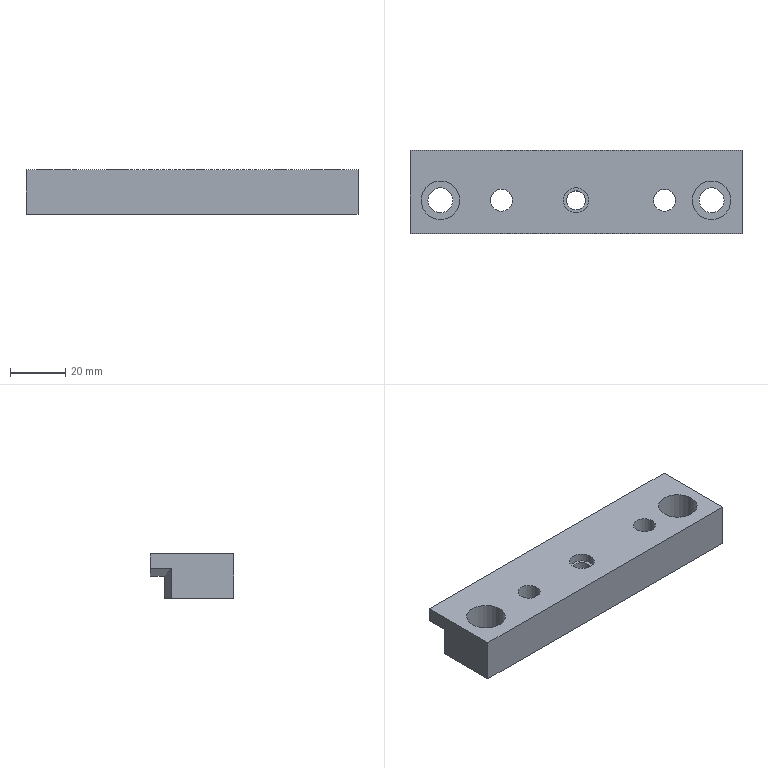Part | STEP file | lll_id730_x_t | 1 solid | 23 faces | box 120 x 30 x 16 mm | volume 46290 mm3 | plane 15 | cylinder 8 | commonest cylinder face diameters 9 x3 8 x2 14 x2 6.8 x1
STEP:
#1=CARTESIAN_POINT('',(1544.035,-355.25,13.));
#2=VERTEX_POINT('',#1);
#3=CARTESIAN_POINT('',(1547.435,-355.25,13.));
#4=DIRECTION('',(0.,0.,1.));
#5=DIRECTION('',(-1.,0.,0.));
#6=AXIS2_PLACEMENT_3D('',#3,#4,#5);
#7=CIRCLE('',#6,3.4);
#8=EDGE_CURVE('',#2,#2,#7,.T.);
#9=ORIENTED_EDGE('',*,*,#8,.F.);
#10=EDGE_LOOP('',(#9));
#11=FACE_BOUND('',#10,.T.);
#12=CARTESIAN_POINT('',(1551.935,-355.25,13.));
#13=VERTEX_POINT('',#12);
#14=CARTESIAN_POINT('',(1547.435,-355.25,13.));
#15=DIRECTION('',(0.,0.,-1.));
#16=DIRECTION('',(1.,0.,0.));
#17=AXIS2_PLACEMENT_3D('',#14,#15,#16);
#18=CIRCLE('',#17,4.5);
#19=EDGE_CURVE('',#13,#13,#18,.T.);
#20=ORIENTED_EDGE('',*,*,#19,.F.);
#21=EDGE_LOOP('',(#20));
#22=FACE_BOUND('',#21,.T.);
#23=CARTESIAN_POINT('',(1547.435,-355.25,13.));
#24=DIRECTION('',(0.,0.,-1.));
#25=DIRECTION('',(-1.,0.,0.));
#26=AXIS2_PLACEMENT_3D('',#23,#24,#25);
#27=PLANE('',#26);
#28=ADVANCED_FACE('',(#11,#22),#27,.F.);
#29=CARTESIAN_POINT('',(1591.935,-355.25,6.));
#30=VERTEX_POINT('',#29);
#31=CARTESIAN_POINT('',(1596.435,-355.25,6.));
#32=DIRECTION('',(0.,0.,1.));
#33=DIRECTION('',(-1.,0.,0.));
#34=AXIS2_PLACEMENT_3D('',#31,#32,#33);
#35=CIRCLE('',#34,4.5);
#36=EDGE_CURVE('',#30,#30,#35,.T.);
#37=ORIENTED_EDGE('',*,*,#36,.F.);
#38=EDGE_LOOP('',(#37));
#39=FACE_BOUND('',#38,.T.);
#40=CARTESIAN_POINT('',(1603.435,-355.25,6.));
#41=VERTEX_POINT('',#40);
#42=CARTESIAN_POINT('',(1596.435,-355.25,6.));
#43=DIRECTION('',(0.,0.,-1.));
#44=DIRECTION('',(1.,0.,0.));
#45=AXIS2_PLACEMENT_3D('',#42,#43,#44);
#46=CIRCLE('',#45,7.);
#47=EDGE_CURVE('',#41,#41,#46,.T.);
#48=ORIENTED_EDGE('',*,*,#47,.F.);
#49=EDGE_LOOP('',(#48));
#50=FACE_BOUND('',#49,.T.);
#51=CARTESIAN_POINT('',(1596.435,-355.25,6.));
#52=DIRECTION('',(0.,0.,-1.));
#53=DIRECTION('',(-1.,0.,0.));
#54=AXIS2_PLACEMENT_3D('',#51,#52,#53);
#55=PLANE('',#54);
#56=ADVANCED_FACE('',(#39,#50),#55,.F.);
#57=CARTESIAN_POINT('',(1597.435,-337.25,8.));
#58=VERTEX_POINT('',#57);
#59=CARTESIAN_POINT('',(1607.435,-337.25,10.679));
#60=VERTEX_POINT('',#59);
#61=CARTESIAN_POINT('',(1607.435,-337.25,10.679));
#62=DIRECTION('',(0.9659,0.,0.2588));
#63=VECTOR('',#62,1.);
#64=LINE('',#61,#63);
#65=EDGE_CURVE('',#58,#60,#64,.T.);
#66=ORIENTED_EDGE('',*,*,#65,.T.);
#67=CARTESIAN_POINT('',(1607.435,-344.929,10.679));
#68=VERTEX_POINT('',#67);
#69=CARTESIAN_POINT('',(1607.435,-337.25,10.679));
#70=DIRECTION('',(0.,-1.,0.));
#71=VECTOR('',#70,1.);
#72=LINE('',#69,#71);
#73=EDGE_CURVE('',#60,#68,#72,.T.);
#74=ORIENTED_EDGE('',*,*,#73,.T.);
#75=CARTESIAN_POINT('',(1597.436,-342.25,8.));
#76=VERTEX_POINT('',#75);
#77=CARTESIAN_POINT('',(1597.436,-342.25,8.));
#78=DIRECTION('',(-0.9351,0.2506,-0.2506));
#79=VECTOR('',#78,1.);
#80=LINE('',#77,#79);
#81=EDGE_CURVE('',#68,#76,#80,.T.);
#82=ORIENTED_EDGE('',*,*,#81,.T.);
#83=CARTESIAN_POINT('',(1597.435,-342.25,8.));
#84=VERTEX_POINT('',#83);
#85=CARTESIAN_POINT('',(1541.456,-342.25,-7.));
#86=DIRECTION('',(-0.9659,0.,-0.2588));
#87=VECTOR('',#86,1.);
#88=LINE('',#85,#87);
#89=EDGE_CURVE('',#76,#84,#88,.T.);
#90=ORIENTED_EDGE('',*,*,#89,.T.);
#91=CARTESIAN_POINT('',(1597.435,-324.452,8.));
#92=DIRECTION('',(0.,1.,0.));
#93=VECTOR('',#92,1.);
#94=LINE('',#91,#93);
#95=EDGE_CURVE('',#84,#58,#94,.T.);
#96=ORIENTED_EDGE('',*,*,#95,.T.);
#97=EDGE_LOOP('',(#66,#74,#82,#90,#96));
#98=FACE_OUTER_BOUND('',#97,.T.);
#99=CARTESIAN_POINT('',(1607.435,-337.25,10.679));
#100=DIRECTION('',(-0.2588,0.,0.9659));
#101=DIRECTION('',(0.9659,0.,0.2588));
#102=AXIS2_PLACEMENT_3D('',#99,#100,#101);
#103=PLANE('',#102);
#104=ADVANCED_FACE('',(#98),#103,.F.);
#105=CARTESIAN_POINT('',(1497.435,-342.251,8.));
#106=VERTEX_POINT('',#105);
#107=CARTESIAN_POINT('',(1487.435,-344.93,10.679));
#108=VERTEX_POINT('',#107);
#109=CARTESIAN_POINT('',(1488.063,-344.762,10.511));
#110=DIRECTION('',(-0.9351,-0.2506,0.2506));
#111=VECTOR('',#110,1.);
#112=LINE('',#109,#111);
#113=EDGE_CURVE('',#106,#108,#112,.T.);
#114=ORIENTED_EDGE('',*,*,#113,.T.);
#115=CARTESIAN_POINT('',(1487.435,-337.25,10.679));
#116=VERTEX_POINT('',#115);
#117=CARTESIAN_POINT('',(1487.435,-367.25,10.679));
#118=DIRECTION('',(0.,1.,0.));
#119=VECTOR('',#118,1.);
#120=LINE('',#117,#119);
#121=EDGE_CURVE('',#108,#116,#120,.T.);
#122=ORIENTED_EDGE('',*,*,#121,.T.);
#123=CARTESIAN_POINT('',(1497.435,-337.25,8.));
#124=VERTEX_POINT('',#123);
#125=CARTESIAN_POINT('',(1487.435,-337.25,10.679));
#126=DIRECTION('',(0.9659,0.,-0.2588));
#127=VECTOR('',#126,1.);
#128=LINE('',#125,#127);
#129=EDGE_CURVE('',#116,#124,#128,.T.);
#130=ORIENTED_EDGE('',*,*,#129,.T.);
#131=CARTESIAN_POINT('',(1497.435,-324.452,8.));
#132=DIRECTION('',(0.,-1.,0.));
#133=VECTOR('',#132,1.);
#134=LINE('',#131,#133);
#135=EDGE_CURVE('',#124,#106,#134,.T.);
#136=ORIENTED_EDGE('',*,*,#135,.T.);
#137=EDGE_LOOP('',(#114,#122,#130,#136));
#138=FACE_OUTER_BOUND('',#137,.T.);
#139=CARTESIAN_POINT('',(1487.435,-367.25,10.679));
#140=DIRECTION('',(0.2588,0.,0.9659));
#141=DIRECTION('',(0.9659,0.,-0.2588));
#142=AXIS2_PLACEMENT_3D('',#139,#140,#141);
#143=PLANE('',#142);
#144=ADVANCED_FACE('',(#138),#143,.F.);
#145=CARTESIAN_POINT('',(1507.435,-337.25,8.));
#146=DIRECTION('',(1.,0.,0.));
#147=VECTOR('',#146,1.);
#148=LINE('',#145,#147);
#149=EDGE_CURVE('',#124,#58,#148,.T.);
#150=ORIENTED_EDGE('',*,*,#149,.T.);
#151=ORIENTED_EDGE('',*,*,#95,.F.);
#152=CARTESIAN_POINT('',(1497.437,-342.25,8.));
#153=VERTEX_POINT('',#152);
#154=CARTESIAN_POINT('',(1517.437,-342.25,8.));
#155=DIRECTION('',(-1.,0.,0.));
#156=VECTOR('',#155,1.);
#157=LINE('',#154,#156);
#158=EDGE_CURVE('',#84,#153,#157,.T.);
#159=ORIENTED_EDGE('',*,*,#158,.T.);
#160=CARTESIAN_POINT('',(1487.435,-344.93,8.));
#161=DIRECTION('',(-0.9659,-0.2588,0.));
#162=VECTOR('',#161,1.);
#163=LINE('',#160,#162);
#164=EDGE_CURVE('',#153,#106,#163,.T.);
#165=ORIENTED_EDGE('',*,*,#164,.T.);
#166=ORIENTED_EDGE('',*,*,#135,.F.);
#167=EDGE_LOOP('',(#150,#151,#159,#165,#166));
#168=FACE_OUTER_BOUND('',#167,.T.);
#169=CARTESIAN_POINT('',(1612.025,-324.452,8.));
#170=DIRECTION('',(0.,0.,1.));
#171=DIRECTION('',(1.,0.,0.));
#172=AXIS2_PLACEMENT_3D('',#169,#170,#171);
#173=PLANE('',#172);
#174=ADVANCED_FACE('',(#168),#173,.F.);
#175=CARTESIAN_POINT('',(1603.435,-355.25,16.));
#176=VERTEX_POINT('',#175);
#177=CARTESIAN_POINT('',(1596.435,-355.25,16.));
#178=DIRECTION('',(0.,0.,-1.));
#179=DIRECTION('',(1.,0.,0.));
#180=AXIS2_PLACEMENT_3D('',#177,#178,#179);
#181=CIRCLE('',#180,7.);
#182=EDGE_CURVE('',#176,#176,#181,.T.);
#183=ORIENTED_EDGE('',*,*,#182,.F.);
#184=EDGE_LOOP('',(#183));
#185=FACE_BOUND('',#184,.T.);
#186=ORIENTED_EDGE('',*,*,#47,.T.);
#187=EDGE_LOOP('',(#186));
#188=FACE_BOUND('',#187,.T.);
#189=CARTESIAN_POINT('',(1596.435,-355.25,47.));
#190=DIRECTION('',(0.,0.,-1.));
#191=DIRECTION('',(-1.,0.,0.));
#192=AXIS2_PLACEMENT_3D('',#189,#190,#191);
#193=CYLINDRICAL_SURFACE('',#192,7.);
#194=ADVANCED_FACE('',(#185,#188),#193,.F.);
#195=CARTESIAN_POINT('',(1487.435,-337.25,16.));
#196=VERTEX_POINT('',#195);
#197=CARTESIAN_POINT('',(1487.435,-337.25,16.));
#198=DIRECTION('',(0.,0.,-1.));
#199=VECTOR('',#198,1.);
#200=LINE('',#197,#199);
#201=EDGE_CURVE('',#196,#116,#200,.T.);
#202=ORIENTED_EDGE('',*,*,#201,.F.);
#203=CARTESIAN_POINT('',(1607.435,-337.25,16.));
#204=VERTEX_POINT('',#203);
#205=CARTESIAN_POINT('',(1507.435,-337.25,16.));
#206=DIRECTION('',(1.,0.,0.));
#207=VECTOR('',#206,1.);
#208=LINE('',#205,#207);
#209=EDGE_CURVE('',#196,#204,#208,.T.);
#210=ORIENTED_EDGE('',*,*,#209,.T.);
#211=CARTESIAN_POINT('',(1607.435,-337.25,16.));
#212=DIRECTION('',(0.,0.,-1.));
#213=VECTOR('',#212,1.);
#214=LINE('',#211,#213);
#215=EDGE_CURVE('',#204,#60,#214,.T.);
#216=ORIENTED_EDGE('',*,*,#215,.T.);
#217=ORIENTED_EDGE('',*,*,#65,.F.);
#218=ORIENTED_EDGE('',*,*,#149,.F.);
#219=ORIENTED_EDGE('',*,*,#129,.F.);
#220=EDGE_LOOP('',(#202,#210,#216,#217,#218,#219));
#221=FACE_OUTER_BOUND('',#220,.T.);
#222=CARTESIAN_POINT('',(1507.435,-337.25,16.));
#223=DIRECTION('',(0.,-1.,0.));
#224=DIRECTION('',(0.,0.,1.));
#225=AXIS2_PLACEMENT_3D('',#222,#223,#224);
#226=PLANE('',#225);
#227=ADVANCED_FACE('',(#221),#226,.F.);
#228=ORIENTED_EDGE('',*,*,#8,.T.);
#229=EDGE_LOOP('',(#228));
#230=FACE_BOUND('',#229,.T.);
#231=CARTESIAN_POINT('',(1550.835,-355.25,0.));
#232=VERTEX_POINT('',#231);
#233=CARTESIAN_POINT('',(1547.435,-355.25,0.));
#234=DIRECTION('',(0.,0.,-1.));
#235=DIRECTION('',(1.,0.,0.));
#236=AXIS2_PLACEMENT_3D('',#233,#234,#235);
#237=CIRCLE('',#236,3.4);
#238=EDGE_CURVE('',#232,#232,#237,.T.);
#239=ORIENTED_EDGE('',*,*,#238,.T.);
#240=EDGE_LOOP('',(#239));
#241=FACE_BOUND('',#240,.T.);
#242=CARTESIAN_POINT('',(1547.435,-355.25,47.));
#243=DIRECTION('',(0.,0.,-1.));
#244=DIRECTION('',(-1.,0.,0.));
#245=AXIS2_PLACEMENT_3D('',#242,#243,#244);
#246=CYLINDRICAL_SURFACE('',#245,3.4);
#247=ADVANCED_FACE('',(#230,#241),#246,.F.);
#248=ORIENTED_EDGE('',*,*,#36,.T.);
#249=EDGE_LOOP('',(#248));
#250=FACE_BOUND('',#249,.T.);
#251=CARTESIAN_POINT('',(1600.935,-355.25,0.));
#252=VERTEX_POINT('',#251);
#253=CARTESIAN_POINT('',(1596.435,-355.25,0.));
#254=DIRECTION('',(0.,0.,-1.));
#255=DIRECTION('',(1.,0.,0.));
#256=AXIS2_PLACEMENT_3D('',#253,#254,#255);
#257=CIRCLE('',#256,4.5);
#258=EDGE_CURVE('',#252,#252,#257,.T.);
#259=ORIENTED_EDGE('',*,*,#258,.T.);
#260=EDGE_LOOP('',(#259));
#261=FACE_BOUND('',#260,.T.);
#262=CARTESIAN_POINT('',(1596.435,-355.25,47.));
#263=DIRECTION('',(0.,0.,-1.));
#264=DIRECTION('',(-1.,0.,0.));
#265=AXIS2_PLACEMENT_3D('',#262,#263,#264);
#266=CYLINDRICAL_SURFACE('',#265,4.5);
#267=ADVANCED_FACE('',(#250,#261),#266,.F.);
#268=CARTESIAN_POINT('',(1497.437,-342.25,0.));
#269=VERTEX_POINT('',#268);
#270=CARTESIAN_POINT('',(1597.436,-342.25,0.));
#271=VERTEX_POINT('',#270);
#272=CARTESIAN_POINT('',(1517.437,-342.25,0.));
#273=DIRECTION('',(1.,0.,0.));
#274=VECTOR('',#273,1.);
#275=LINE('',#272,#274);
#276=EDGE_CURVE('',#269,#271,#275,.T.);
#277=ORIENTED_EDGE('',*,*,#276,.F.);
#278=CARTESIAN_POINT('',(1497.437,-342.25,8.));
#279=DIRECTION('',(0.,0.,1.));
#280=VECTOR('',#279,1.);
#281=LINE('',#278,#280);
#282=EDGE_CURVE('',#269,#153,#281,.T.);
#283=ORIENTED_EDGE('',*,*,#282,.T.);
#284=ORIENTED_EDGE('',*,*,#158,.F.);
#285=ORIENTED_EDGE('',*,*,#89,.F.);
#286=CARTESIAN_POINT('',(1597.436,-342.25,8.));
#287=DIRECTION('',(0.,0.,1.));
#288=VECTOR('',#287,1.);
#289=LINE('',#286,#288);
#290=EDGE_CURVE('',#271,#76,#289,.T.);
#291=ORIENTED_EDGE('',*,*,#290,.F.);
#292=EDGE_LOOP('',(#277,#283,#284,#285,#291));
#293=FACE_OUTER_BOUND('',#292,.T.);
#294=CARTESIAN_POINT('',(1517.437,-342.25,8.));
#295=DIRECTION('',(0.,-1.,0.));
#296=DIRECTION('',(0.,0.,1.));
#297=AXIS2_PLACEMENT_3D('',#294,#295,#296);
#298=PLANE('',#297);
#299=ADVANCED_FACE('',(#293),#298,.F.);
#300=CARTESIAN_POINT('',(1607.435,-344.929,0.));
#301=VERTEX_POINT('',#300);
#302=CARTESIAN_POINT('',(1597.436,-342.25,0.));
#303=DIRECTION('',(0.9659,-0.2588,0.));
#304=VECTOR('',#303,1.);
#305=LINE('',#302,#304);
#306=EDGE_CURVE('',#271,#301,#305,.T.);
#307=ORIENTED_EDGE('',*,*,#306,.F.);
#308=ORIENTED_EDGE('',*,*,#290,.T.);
#309=ORIENTED_EDGE('',*,*,#81,.F.);
#310=CARTESIAN_POINT('',(1607.435,-344.929,8.));
#311=DIRECTION('',(0.,0.,-1.));
#312=VECTOR('',#311,1.);
#313=LINE('',#310,#312);
#314=EDGE_CURVE('',#68,#301,#313,.T.);
#315=ORIENTED_EDGE('',*,*,#314,.T.);
#316=EDGE_LOOP('',(#307,#308,#309,#315));
#317=FACE_OUTER_BOUND('',#316,.T.);
#318=CARTESIAN_POINT('',(1597.436,-342.25,8.));
#319=DIRECTION('',(-0.2588,-0.9659,0.));
#320=DIRECTION('',(-0.9659,0.2588,0.));
#321=AXIS2_PLACEMENT_3D('',#318,#319,#320);
#322=PLANE('',#321);
#323=ADVANCED_FACE('',(#317),#322,.F.);
#324=ORIENTED_EDGE('',*,*,#215,.F.);
#325=CARTESIAN_POINT('',(1607.435,-367.25,16.));
#326=VERTEX_POINT('',#325);
#327=CARTESIAN_POINT('',(1607.435,-337.25,16.));
#328=DIRECTION('',(0.,-1.,0.));
#329=VECTOR('',#328,1.);
#330=LINE('',#327,#329);
#331=EDGE_CURVE('',#204,#326,#330,.T.);
#332=ORIENTED_EDGE('',*,*,#331,.T.);
#333=CARTESIAN_POINT('',(1607.435,-367.25,0.));
#334=VERTEX_POINT('',#333);
#335=CARTESIAN_POINT('',(1607.435,-367.25,16.));
#336=DIRECTION('',(0.,0.,-1.));
#337=VECTOR('',#336,1.);
#338=LINE('',#335,#337);
#339=EDGE_CURVE('',#326,#334,#338,.T.);
#340=ORIENTED_EDGE('',*,*,#339,.T.);
#341=CARTESIAN_POINT('',(1607.435,-337.25,0.));
#342=DIRECTION('',(0.,-1.,0.));
#343=VECTOR('',#342,1.);
#344=LINE('',#341,#343);
#345=EDGE_CURVE('',#301,#334,#344,.T.);
#346=ORIENTED_EDGE('',*,*,#345,.F.);
#347=ORIENTED_EDGE('',*,*,#314,.F.);
#348=ORIENTED_EDGE('',*,*,#73,.F.);
#349=EDGE_LOOP('',(#324,#332,#340,#346,#347,#348));
#350=FACE_OUTER_BOUND('',#349,.T.);
#351=CARTESIAN_POINT('',(1607.435,-337.25,16.));
#352=DIRECTION('',(-1.,0.,0.));
#353=DIRECTION('',(0.,0.,1.));
#354=AXIS2_PLACEMENT_3D('',#351,#352,#353);
#355=PLANE('',#354);
#356=ADVANCED_FACE('',(#350),#355,.F.);
#357=CARTESIAN_POINT('',(1487.435,-367.25,0.));
#358=VERTEX_POINT('',#357);
#359=CARTESIAN_POINT('',(1587.435,-367.25,0.));
#360=DIRECTION('',(-1.,0.,0.));
#361=VECTOR('',#360,1.);
#362=LINE('',#359,#361);
#363=EDGE_CURVE('',#334,#358,#362,.T.);
#364=ORIENTED_EDGE('',*,*,#363,.F.);
#365=ORIENTED_EDGE('',*,*,#339,.F.);
#366=CARTESIAN_POINT('',(1487.435,-367.25,16.));
#367=VERTEX_POINT('',#366);
#368=CARTESIAN_POINT('',(1587.435,-367.25,16.));
#369=DIRECTION('',(-1.,0.,0.));
#370=VECTOR('',#369,1.);
#371=LINE('',#368,#370);
#372=EDGE_CURVE('',#326,#367,#371,.T.);
#373=ORIENTED_EDGE('',*,*,#372,.T.);
#374=CARTESIAN_POINT('',(1487.435,-367.25,16.));
#375=DIRECTION('',(0.,0.,-1.));
#376=VECTOR('',#375,1.);
#377=LINE('',#374,#376);
#378=EDGE_CURVE('',#367,#358,#377,.T.);
#379=ORIENTED_EDGE('',*,*,#378,.T.);
#380=EDGE_LOOP('',(#364,#365,#373,#379));
#381=FACE_OUTER_BOUND('',#380,.T.);
#382=CARTESIAN_POINT('',(1587.435,-367.25,16.));
#383=DIRECTION('',(0.,1.,0.));
#384=DIRECTION('',(0.,0.,-1.));
#385=AXIS2_PLACEMENT_3D('',#382,#383,#384);
#386=PLANE('',#385);
#387=ADVANCED_FACE('',(#381),#386,.F.);
#388=CARTESIAN_POINT('',(1487.435,-344.93,0.));
#389=VERTEX_POINT('',#388);
#390=CARTESIAN_POINT('',(1487.435,-344.93,8.));
#391=DIRECTION('',(0.,0.,-1.));
#392=VECTOR('',#391,1.);
#393=LINE('',#390,#392);
#394=EDGE_CURVE('',#108,#389,#393,.T.);
#395=ORIENTED_EDGE('',*,*,#394,.T.);
#396=CARTESIAN_POINT('',(1487.435,-367.25,0.));
#397=DIRECTION('',(0.,1.,0.));
#398=VECTOR('',#397,1.);
#399=LINE('',#396,#398);
#400=EDGE_CURVE('',#358,#389,#399,.T.);
#401=ORIENTED_EDGE('',*,*,#400,.F.);
#402=ORIENTED_EDGE('',*,*,#378,.F.);
#403=CARTESIAN_POINT('',(1487.435,-367.25,16.));
#404=DIRECTION('',(0.,1.,0.));
#405=VECTOR('',#404,1.);
#406=LINE('',#403,#405);
#407=EDGE_CURVE('',#367,#196,#406,.T.);
#408=ORIENTED_EDGE('',*,*,#407,.T.);
#409=ORIENTED_EDGE('',*,*,#201,.T.);
#410=ORIENTED_EDGE('',*,*,#121,.F.);
#411=EDGE_LOOP('',(#395,#401,#402,#408,#409,#410));
#412=FACE_OUTER_BOUND('',#411,.T.);
#413=CARTESIAN_POINT('',(1487.435,-367.25,16.));
#414=DIRECTION('',(1.,0.,0.));
#415=DIRECTION('',(0.,0.,-1.));
#416=AXIS2_PLACEMENT_3D('',#413,#414,#415);
#417=PLANE('',#416);
#418=ADVANCED_FACE('',(#412),#417,.F.);
#419=CARTESIAN_POINT('',(1487.435,-344.93,0.));
#420=DIRECTION('',(0.9659,0.2588,0.));
#421=VECTOR('',#420,1.);
#422=LINE('',#419,#421);
#423=EDGE_CURVE('',#389,#269,#422,.T.);
#424=ORIENTED_EDGE('',*,*,#423,.F.);
#425=ORIENTED_EDGE('',*,*,#394,.F.);
#426=ORIENTED_EDGE('',*,*,#113,.F.);
#427=ORIENTED_EDGE('',*,*,#164,.F.);
#428=ORIENTED_EDGE('',*,*,#282,.F.);
#429=EDGE_LOOP('',(#424,#425,#426,#427,#428));
#430=FACE_OUTER_BOUND('',#429,.T.);
#431=CARTESIAN_POINT('',(1487.435,-344.93,8.));
#432=DIRECTION('',(0.2588,-0.9659,0.));
#433=DIRECTION('',(-0.9659,-0.2588,0.));
#434=AXIS2_PLACEMENT_3D('',#431,#432,#433);
#435=PLANE('',#434);
#436=ADVANCED_FACE('',(#430),#435,.F.);
#437=CARTESIAN_POINT('',(1583.435,-355.25,16.));
#438=VERTEX_POINT('',#437);
#439=CARTESIAN_POINT('',(1579.435,-355.25,16.));
#440=DIRECTION('',(0.,0.,1.));
#441=DIRECTION('',(1.,0.,0.));
#442=AXIS2_PLACEMENT_3D('',#439,#440,#441);
#443=CIRCLE('',#442,4.);
#444=EDGE_CURVE('',#438,#438,#443,.T.);
#445=ORIENTED_EDGE('',*,*,#444,.T.);
#446=EDGE_LOOP('',(#445));
#447=FACE_BOUND('',#446,.T.);
#448=CARTESIAN_POINT('',(1583.435,-355.25,0.));
#449=VERTEX_POINT('',#448);
#450=CARTESIAN_POINT('',(1579.435,-355.25,0.));
#451=DIRECTION('',(0.,0.,-1.));
#452=DIRECTION('',(1.,0.,0.));
#453=AXIS2_PLACEMENT_3D('',#450,#451,#452);
#454=CIRCLE('',#453,4.);
#455=EDGE_CURVE('',#449,#449,#454,.T.);
#456=ORIENTED_EDGE('',*,*,#455,.T.);
#457=EDGE_LOOP('',(#456));
#458=FACE_BOUND('',#457,.T.);
#459=CARTESIAN_POINT('',(1579.435,-355.25,47.));
#460=DIRECTION('',(0.,0.,-1.));
#461=DIRECTION('',(-1.,0.,0.));
#462=AXIS2_PLACEMENT_3D('',#459,#460,#461);
#463=CYLINDRICAL_SURFACE('',#462,4.);
#464=ADVANCED_FACE('',(#447,#458),#463,.F.);
#465=CARTESIAN_POINT('',(1524.435,-355.25,0.));
#466=VERTEX_POINT('',#465);
#467=CARTESIAN_POINT('',(1520.435,-355.25,0.));
#468=DIRECTION('',(0.,0.,1.));
#469=DIRECTION('',(1.,0.,0.));
#470=AXIS2_PLACEMENT_3D('',#467,#468,#469);
#471=CIRCLE('',#470,4.);
#472=EDGE_CURVE('',#466,#466,#471,.T.);
#473=ORIENTED_EDGE('',*,*,#472,.T.);
#474=EDGE_LOOP('',(#473));
#475=FACE_BOUND('',#474,.T.);
#476=ORIENTED_EDGE('',*,*,#455,.F.);
#477=EDGE_LOOP('',(#476));
#478=FACE_BOUND('',#477,.T.);
#479=ORIENTED_EDGE('',*,*,#423,.T.);
#480=ORIENTED_EDGE('',*,*,#276,.T.);
#481=ORIENTED_EDGE('',*,*,#306,.T.);
#482=ORIENTED_EDGE('',*,*,#345,.T.);
#483=ORIENTED_EDGE('',*,*,#363,.T.);
#484=ORIENTED_EDGE('',*,*,#400,.T.);
#485=EDGE_LOOP('',(#479,#480,#481,#482,#483,#484));
#486=FACE_BOUND('',#485,.T.);
#487=ORIENTED_EDGE('',*,*,#258,.F.);
#488=EDGE_LOOP('',(#487));
#489=FACE_BOUND('',#488,.T.);
#490=ORIENTED_EDGE('',*,*,#238,.F.);
#491=EDGE_LOOP('',(#490));
#492=FACE_BOUND('',#491,.T.);
#493=CARTESIAN_POINT('',(1502.935,-355.25,0.));
#494=VERTEX_POINT('',#493);
#495=CARTESIAN_POINT('',(1498.435,-355.25,0.));
#496=DIRECTION('',(0.,0.,1.));
#497=DIRECTION('',(1.,0.,0.));
#498=AXIS2_PLACEMENT_3D('',#495,#496,#497);
#499=CIRCLE('',#498,4.5);
#500=EDGE_CURVE('',#494,#494,#499,.T.);
#501=ORIENTED_EDGE('',*,*,#500,.T.);
#502=EDGE_LOOP('',(#501));
#503=FACE_BOUND('',#502,.T.);
#504=CARTESIAN_POINT('',(1507.435,-367.25,0.));
#505=DIRECTION('',(0.,0.,1.));
#506=DIRECTION('',(1.,0.,0.));
#507=AXIS2_PLACEMENT_3D('',#504,#505,#506);
#508=PLANE('',#507);
#509=ADVANCED_FACE('',(#475,#478,#486,#489,#492,#503),#508,.F.);
#510=CARTESIAN_POINT('',(1551.935,-355.25,16.));
#511=VERTEX_POINT('',#510);
#512=CARTESIAN_POINT('',(1547.435,-355.25,16.));
#513=DIRECTION('',(0.,0.,-1.));
#514=DIRECTION('',(1.,0.,0.));
#515=AXIS2_PLACEMENT_3D('',#512,#513,#514);
#516=CIRCLE('',#515,4.5);
#517=EDGE_CURVE('',#511,#511,#516,.T.);
#518=ORIENTED_EDGE('',*,*,#517,.F.);
#519=EDGE_LOOP('',(#518));
#520=FACE_BOUND('',#519,.T.);
#521=ORIENTED_EDGE('',*,*,#19,.T.);
#522=EDGE_LOOP('',(#521));
#523=FACE_BOUND('',#522,.T.);
#524=CARTESIAN_POINT('',(1547.435,-355.25,47.));
#525=DIRECTION('',(0.,0.,-1.));
#526=DIRECTION('',(-1.,0.,0.));
#527=AXIS2_PLACEMENT_3D('',#524,#525,#526);
#528=CYLINDRICAL_SURFACE('',#527,4.5);
#529=ADVANCED_FACE('',(#520,#523),#528,.F.);
#530=CARTESIAN_POINT('',(1505.435,-355.25,16.));
#531=VERTEX_POINT('',#530);
#532=CARTESIAN_POINT('',(1498.435,-355.25,16.));
#533=DIRECTION('',(0.,0.,-1.));
#534=DIRECTION('',(1.,0.,0.));
#535=AXIS2_PLACEMENT_3D('',#532,#533,#534);
#536=CIRCLE('',#535,7.);
#537=EDGE_CURVE('',#531,#531,#536,.T.);
#538=ORIENTED_EDGE('',*,*,#537,.T.);
#539=EDGE_LOOP('',(#538));
#540=FACE_BOUND('',#539,.T.);
#541=ORIENTED_EDGE('',*,*,#517,.T.);
#542=EDGE_LOOP('',(#541));
#543=FACE_BOUND('',#542,.T.);
#544=ORIENTED_EDGE('',*,*,#372,.F.);
#545=ORIENTED_EDGE('',*,*,#331,.F.);
#546=ORIENTED_EDGE('',*,*,#209,.F.);
#547=ORIENTED_EDGE('',*,*,#407,.F.);
#548=EDGE_LOOP('',(#544,#545,#546,#547));
#549=FACE_BOUND('',#548,.T.);
#550=ORIENTED_EDGE('',*,*,#444,.F.);
#551=EDGE_LOOP('',(#550));
#552=FACE_BOUND('',#551,.T.);
#553=ORIENTED_EDGE('',*,*,#182,.T.);
#554=EDGE_LOOP('',(#553));
#555=FACE_BOUND('',#554,.T.);
#556=CARTESIAN_POINT('',(1524.435,-355.25,16.));
#557=VERTEX_POINT('',#556);
#558=CARTESIAN_POINT('',(1520.435,-355.25,16.));
#559=DIRECTION('',(0.,0.,1.));
#560=DIRECTION('',(1.,0.,0.));
#561=AXIS2_PLACEMENT_3D('',#558,#559,#560);
#562=CIRCLE('',#561,4.);
#563=EDGE_CURVE('',#557,#557,#562,.T.);
#564=ORIENTED_EDGE('',*,*,#563,.F.);
#565=EDGE_LOOP('',(#564));
#566=FACE_BOUND('',#565,.T.);
#567=CARTESIAN_POINT('',(1507.435,-367.25,16.));
#568=DIRECTION('',(0.,0.,1.));
#569=DIRECTION('',(1.,0.,0.));
#570=AXIS2_PLACEMENT_3D('',#567,#568,#569);
#571=PLANE('',#570);
#572=ADVANCED_FACE('',(#540,#543,#549,#552,#555,#566),#571,.T.);
#573=ORIENTED_EDGE('',*,*,#563,.T.);
#574=EDGE_LOOP('',(#573));
#575=FACE_BOUND('',#574,.T.);
#576=ORIENTED_EDGE('',*,*,#472,.F.);
#577=EDGE_LOOP('',(#576));
#578=FACE_BOUND('',#577,.T.);
#579=CARTESIAN_POINT('',(1520.435,-355.25,47.));
#580=DIRECTION('',(0.,0.,-1.));
#581=DIRECTION('',(1.,0.,0.));
#582=AXIS2_PLACEMENT_3D('',#579,#580,#581);
#583=CYLINDRICAL_SURFACE('',#582,4.);
#584=ADVANCED_FACE('',(#575,#578),#583,.F.);
#585=CARTESIAN_POINT('',(1502.935,-355.25,6.));
#586=VERTEX_POINT('',#585);
#587=CARTESIAN_POINT('',(1498.435,-355.25,6.));
#588=DIRECTION('',(0.,0.,1.));
#589=DIRECTION('',(1.,0.,0.));
#590=AXIS2_PLACEMENT_3D('',#587,#588,#589);
#591=CIRCLE('',#590,4.5);
#592=EDGE_CURVE('',#586,#586,#591,.T.);
#593=ORIENTED_EDGE('',*,*,#592,.F.);
#594=EDGE_LOOP('',(#593));
#595=FACE_BOUND('',#594,.T.);
#596=CARTESIAN_POINT('',(1491.435,-355.25,6.));
#597=VERTEX_POINT('',#596);
#598=CARTESIAN_POINT('',(1498.435,-355.25,6.));
#599=DIRECTION('',(0.,0.,-1.));
#600=DIRECTION('',(-1.,0.,0.));
#601=AXIS2_PLACEMENT_3D('',#598,#599,#600);
#602=CIRCLE('',#601,7.);
#603=EDGE_CURVE('',#597,#597,#602,.T.);
#604=ORIENTED_EDGE('',*,*,#603,.F.);
#605=EDGE_LOOP('',(#604));
#606=FACE_BOUND('',#605,.T.);
#607=CARTESIAN_POINT('',(1498.435,-355.25,6.));
#608=DIRECTION('',(0.,0.,-1.));
#609=DIRECTION('',(1.,0.,0.));
#610=AXIS2_PLACEMENT_3D('',#607,#608,#609);
#611=PLANE('',#610);
#612=ADVANCED_FACE('',(#595,#606),#611,.F.);
#613=ORIENTED_EDGE('',*,*,#592,.T.);
#614=EDGE_LOOP('',(#613));
#615=FACE_BOUND('',#614,.T.);
#616=ORIENTED_EDGE('',*,*,#500,.F.);
#617=EDGE_LOOP('',(#616));
#618=FACE_BOUND('',#617,.T.);
#619=CARTESIAN_POINT('',(1498.435,-355.25,47.));
#620=DIRECTION('',(0.,0.,-1.));
#621=DIRECTION('',(1.,0.,0.));
#622=AXIS2_PLACEMENT_3D('',#619,#620,#621);
#623=CYLINDRICAL_SURFACE('',#622,4.5);
#624=ADVANCED_FACE('',(#615,#618),#623,.F.);
#625=ORIENTED_EDGE('',*,*,#537,.F.);
#626=EDGE_LOOP('',(#625));
#627=FACE_BOUND('',#626,.T.);
#628=ORIENTED_EDGE('',*,*,#603,.T.);
#629=EDGE_LOOP('',(#628));
#630=FACE_BOUND('',#629,.T.);
#631=CARTESIAN_POINT('',(1498.435,-355.25,47.));
#632=DIRECTION('',(0.,0.,-1.));
#633=DIRECTION('',(1.,0.,0.));
#634=AXIS2_PLACEMENT_3D('',#631,#632,#633);
#635=CYLINDRICAL_SURFACE('',#634,7.);
#636=ADVANCED_FACE('',(#627,#630),#635,.F.);
#637=CLOSED_SHELL('',(#28,#56,#104,#144,#174,#194,#227,#247,#267,#299,#323,#356,#387,#418,#436,#464,#509,#529,#572,#584,#612,#624,#636));
#638=MANIFOLD_SOLID_BREP('',#637);
#639=(LENGTH_UNIT()NAMED_UNIT(*)SI_UNIT(.MILLI.,.METRE.));
#640=UNCERTAINTY_MEASURE_WITH_UNIT(LENGTH_MEASURE(0.00002),#639,'','');
#641=(NAMED_UNIT(*)PLANE_ANGLE_UNIT()SI_UNIT($,.RADIAN.));
#642=PLANE_ANGLE_MEASURE_WITH_UNIT(PLANE_ANGLE_MEASURE(0.01745),#641);
#643=DIMENSIONAL_EXPONENTS(0.,0.,0.,0.,0.,0.,0.);
#644=(CONVERSION_BASED_UNIT('DEGREE',#642)NAMED_UNIT(#643)PLANE_ANGLE_UNIT());
#645=(NAMED_UNIT(*)SI_UNIT($,.STERADIAN.)SOLID_ANGLE_UNIT());
#646=(GEOMETRIC_REPRESENTATION_CONTEXT(3)GLOBAL_UNCERTAINTY_ASSIGNED_CONTEXT((#640))GLOBAL_UNIT_ASSIGNED_CONTEXT((#639,#644,#645))REPRESENTATION_CONTEXT('',''));
#647=ADVANCED_BREP_SHAPE_REPRESENTATION('',(#638),#646);